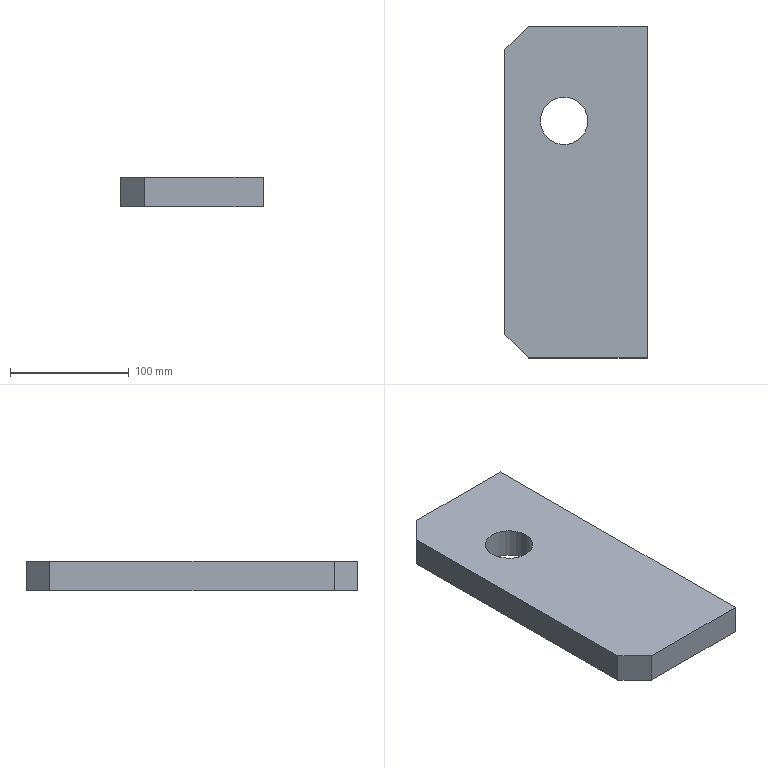Part | SolidWorks | features Chamfer 1, Extrusion 1, ICE 1 | 1 solid | 10 faces | box 120 x 280 x 25 mm | volume 798584 mm3 | plane 8 | cylinder 2 | commonest cylinder face diameters 40 x2
STEP:
#1=CARTESIAN_POINT('',(-90.,200.,0.));
#2=VERTEX_POINT('',#1);
#3=CARTESIAN_POINT('',(-50.,200.,0.));
#4=VERTEX_POINT('',#3);
#5=CARTESIAN_POINT('',(-70.,200.,0.));
#6=DIRECTION('',(0.,0.,1.));
#7=DIRECTION('',(1.,0.,0.));
#8=AXIS2_PLACEMENT_3D('',#5,#6,#7);
#9=CIRCLE('',#8,20.);
#10=EDGE_CURVE('',#2,#4,#9,.T.);
#11=ORIENTED_EDGE('',*,*,#10,.F.);
#12=CARTESIAN_POINT('',(-90.,200.,25.));
#13=VERTEX_POINT('',#12);
#14=CARTESIAN_POINT('',(-90.,200.,0.));
#15=DIRECTION('',(0.,0.,1.));
#16=VECTOR('',#15,1000.);
#17=LINE('',#14,#16);
#18=EDGE_CURVE('',#2,#13,#17,.T.);
#19=ORIENTED_EDGE('',*,*,#18,.T.);
#20=CARTESIAN_POINT('',(-50.,200.,25.));
#21=VERTEX_POINT('',#20);
#22=CARTESIAN_POINT('',(-70.,200.,25.));
#23=DIRECTION('',(0.,0.,1.));
#24=DIRECTION('',(1.,0.,0.));
#25=AXIS2_PLACEMENT_3D('',#22,#23,#24);
#26=CIRCLE('',#25,20.);
#27=EDGE_CURVE('',#13,#21,#26,.T.);
#28=ORIENTED_EDGE('',*,*,#27,.T.);
#29=CARTESIAN_POINT('',(-50.,200.,0.));
#30=DIRECTION('',(0.,0.,1.));
#31=VECTOR('',#30,1000.);
#32=LINE('',#29,#31);
#33=EDGE_CURVE('',#4,#21,#32,.T.);
#34=ORIENTED_EDGE('',*,*,#33,.F.);
#35=EDGE_LOOP('',(#11,#19,#28,#34));
#36=FACE_OUTER_BOUND('',#35,.T.);
#37=CARTESIAN_POINT('',(-70.,200.,0.));
#38=DIRECTION('',(0.,0.,1.));
#39=DIRECTION('',(1.,0.,0.));
#40=AXIS2_PLACEMENT_3D('',#37,#38,#39);
#41=CYLINDRICAL_SURFACE('',#40,20.);
#42=ADVANCED_FACE('',(#36),#41,.F.);
#43=CARTESIAN_POINT('',(0.,0.,0.));
#44=VERTEX_POINT('',#43);
#45=CARTESIAN_POINT('',(0.,280.,0.));
#46=VERTEX_POINT('',#45);
#47=CARTESIAN_POINT('',(0.,0.,0.));
#48=DIRECTION('',(0.,1.,0.));
#49=VECTOR('',#48,1000.);
#50=LINE('',#47,#49);
#51=EDGE_CURVE('',#44,#46,#50,.T.);
#52=ORIENTED_EDGE('',*,*,#51,.T.);
#53=CARTESIAN_POINT('',(0.,280.,25.));
#54=VERTEX_POINT('',#53);
#55=CARTESIAN_POINT('',(0.,280.,25.));
#56=DIRECTION('',(0.,0.,-1.));
#57=VECTOR('',#56,1000.);
#58=LINE('',#55,#57);
#59=EDGE_CURVE('',#54,#46,#58,.T.);
#60=ORIENTED_EDGE('',*,*,#59,.F.);
#61=CARTESIAN_POINT('',(0.,0.,25.));
#62=VERTEX_POINT('',#61);
#63=CARTESIAN_POINT('',(0.,0.,25.));
#64=DIRECTION('',(0.,1.,0.));
#65=VECTOR('',#64,1000.);
#66=LINE('',#63,#65);
#67=EDGE_CURVE('',#62,#54,#66,.T.);
#68=ORIENTED_EDGE('',*,*,#67,.F.);
#69=CARTESIAN_POINT('',(0.,0.,25.));
#70=DIRECTION('',(0.,0.,-1.));
#71=VECTOR('',#70,1000.);
#72=LINE('',#69,#71);
#73=EDGE_CURVE('',#62,#44,#72,.T.);
#74=ORIENTED_EDGE('',*,*,#73,.T.);
#75=EDGE_LOOP('',(#52,#60,#68,#74));
#76=FACE_OUTER_BOUND('',#75,.T.);
#77=CARTESIAN_POINT('',(0.,0.,25.));
#78=DIRECTION('',(-1.,0.,0.));
#79=DIRECTION('',(0.,0.,1.));
#80=AXIS2_PLACEMENT_3D('',#77,#78,#79);
#81=PLANE('',#80);
#82=ADVANCED_FACE('',(#76),#81,.F.);
#83=CARTESIAN_POINT('',(-100.,280.,0.));
#84=VERTEX_POINT('',#83);
#85=CARTESIAN_POINT('',(0.,280.,0.));
#86=DIRECTION('',(-1.,0.,0.));
#87=VECTOR('',#86,1000.);
#88=LINE('',#85,#87);
#89=EDGE_CURVE('',#46,#84,#88,.T.);
#90=ORIENTED_EDGE('',*,*,#89,.T.);
#91=CARTESIAN_POINT('',(-100.,280.,25.));
#92=VERTEX_POINT('',#91);
#93=CARTESIAN_POINT('',(-100.,280.,25.));
#94=DIRECTION('',(0.,0.,1.));
#95=VECTOR('',#94,1000.);
#96=LINE('',#93,#95);
#97=EDGE_CURVE('',#84,#92,#96,.T.);
#98=ORIENTED_EDGE('',*,*,#97,.T.);
#99=CARTESIAN_POINT('',(0.,280.,25.));
#100=DIRECTION('',(-1.,0.,0.));
#101=VECTOR('',#100,1000.);
#102=LINE('',#99,#101);
#103=EDGE_CURVE('',#54,#92,#102,.T.);
#104=ORIENTED_EDGE('',*,*,#103,.F.);
#105=ORIENTED_EDGE('',*,*,#59,.T.);
#106=EDGE_LOOP('',(#90,#98,#104,#105));
#107=FACE_OUTER_BOUND('',#106,.T.);
#108=CARTESIAN_POINT('',(0.,280.,25.));
#109=DIRECTION('',(0.,-1.,0.));
#110=DIRECTION('',(0.,0.,-1.));
#111=AXIS2_PLACEMENT_3D('',#108,#109,#110);
#112=PLANE('',#111);
#113=ADVANCED_FACE('',(#107),#112,.F.);
#114=CARTESIAN_POINT('',(-120.,260.,0.));
#115=VERTEX_POINT('',#114);
#116=CARTESIAN_POINT('',(-120.,20.,0.));
#117=VERTEX_POINT('',#116);
#118=CARTESIAN_POINT('',(-120.,0.,0.));
#119=DIRECTION('',(0.,-1.,0.));
#120=VECTOR('',#119,1000.);
#121=LINE('',#118,#120);
#122=EDGE_CURVE('',#115,#117,#121,.T.);
#123=ORIENTED_EDGE('',*,*,#122,.T.);
#124=CARTESIAN_POINT('',(-120.,20.,25.));
#125=VERTEX_POINT('',#124);
#126=CARTESIAN_POINT('',(-120.,20.,25.));
#127=DIRECTION('',(0.,0.,1.));
#128=VECTOR('',#127,1000.);
#129=LINE('',#126,#128);
#130=EDGE_CURVE('',#117,#125,#129,.T.);
#131=ORIENTED_EDGE('',*,*,#130,.T.);
#132=CARTESIAN_POINT('',(-120.,260.,25.));
#133=VERTEX_POINT('',#132);
#134=CARTESIAN_POINT('',(-120.,0.,25.));
#135=DIRECTION('',(0.,-1.,0.));
#136=VECTOR('',#135,1000.);
#137=LINE('',#134,#136);
#138=EDGE_CURVE('',#133,#125,#137,.T.);
#139=ORIENTED_EDGE('',*,*,#138,.F.);
#140=CARTESIAN_POINT('',(-120.,260.,25.));
#141=DIRECTION('',(0.,0.,-1.));
#142=VECTOR('',#141,1000.);
#143=LINE('',#140,#142);
#144=EDGE_CURVE('',#133,#115,#143,.T.);
#145=ORIENTED_EDGE('',*,*,#144,.T.);
#146=EDGE_LOOP('',(#123,#131,#139,#145));
#147=FACE_OUTER_BOUND('',#146,.T.);
#148=CARTESIAN_POINT('',(-120.,0.,25.));
#149=DIRECTION('',(1.,0.,0.));
#150=DIRECTION('',(0.,0.,-1.));
#151=AXIS2_PLACEMENT_3D('',#148,#149,#150);
#152=PLANE('',#151);
#153=ADVANCED_FACE('',(#147),#152,.F.);
#154=CARTESIAN_POINT('',(-100.,0.,25.));
#155=VERTEX_POINT('',#154);
#156=CARTESIAN_POINT('',(0.,0.,25.));
#157=DIRECTION('',(1.,0.,0.));
#158=VECTOR('',#157,1000.);
#159=LINE('',#156,#158);
#160=EDGE_CURVE('',#155,#62,#159,.T.);
#161=ORIENTED_EDGE('',*,*,#160,.F.);
#162=CARTESIAN_POINT('',(-100.,0.,0.));
#163=VERTEX_POINT('',#162);
#164=CARTESIAN_POINT('',(-100.,0.,25.));
#165=DIRECTION('',(0.,0.,-1.));
#166=VECTOR('',#165,1000.);
#167=LINE('',#164,#166);
#168=EDGE_CURVE('',#155,#163,#167,.T.);
#169=ORIENTED_EDGE('',*,*,#168,.T.);
#170=CARTESIAN_POINT('',(0.,0.,0.));
#171=DIRECTION('',(1.,0.,0.));
#172=VECTOR('',#171,1000.);
#173=LINE('',#170,#172);
#174=EDGE_CURVE('',#163,#44,#173,.T.);
#175=ORIENTED_EDGE('',*,*,#174,.T.);
#176=ORIENTED_EDGE('',*,*,#73,.F.);
#177=EDGE_LOOP('',(#161,#169,#175,#176));
#178=FACE_OUTER_BOUND('',#177,.T.);
#179=CARTESIAN_POINT('',(0.,0.,25.));
#180=DIRECTION('',(0.,1.,0.));
#181=DIRECTION('',(0.,0.,1.));
#182=AXIS2_PLACEMENT_3D('',#179,#180,#181);
#183=PLANE('',#182);
#184=ADVANCED_FACE('',(#178),#183,.F.);
#185=CARTESIAN_POINT('',(-70.,200.,25.));
#186=DIRECTION('',(0.,0.,1.));
#187=DIRECTION('',(1.,0.,0.));
#188=AXIS2_PLACEMENT_3D('',#185,#186,#187);
#189=CIRCLE('',#188,20.);
#190=EDGE_CURVE('',#21,#13,#189,.T.);
#191=ORIENTED_EDGE('',*,*,#190,.F.);
#192=ORIENTED_EDGE('',*,*,#27,.F.);
#193=EDGE_LOOP('',(#191,#192));
#194=FACE_BOUND('',#193,.T.);
#195=ORIENTED_EDGE('',*,*,#138,.T.);
#196=CARTESIAN_POINT('',(-50.,-50.,25.));
#197=DIRECTION('',(0.7071,-0.7071,0.));
#198=VECTOR('',#197,1000.);
#199=LINE('',#196,#198);
#200=EDGE_CURVE('',#125,#155,#199,.T.);
#201=ORIENTED_EDGE('',*,*,#200,.T.);
#202=ORIENTED_EDGE('',*,*,#160,.T.);
#203=ORIENTED_EDGE('',*,*,#67,.T.);
#204=ORIENTED_EDGE('',*,*,#103,.T.);
#205=CARTESIAN_POINT('',(-190.,190.,25.));
#206=DIRECTION('',(-0.7071,-0.7071,0.));
#207=VECTOR('',#206,1000.);
#208=LINE('',#205,#207);
#209=EDGE_CURVE('',#92,#133,#208,.T.);
#210=ORIENTED_EDGE('',*,*,#209,.T.);
#211=EDGE_LOOP('',(#195,#201,#202,#203,#204,#210));
#212=FACE_OUTER_BOUND('',#211,.T.);
#213=CARTESIAN_POINT('',(0.,0.,25.));
#214=DIRECTION('',(0.,0.,1.));
#215=DIRECTION('',(1.,0.,0.));
#216=AXIS2_PLACEMENT_3D('',#213,#214,#215);
#217=PLANE('',#216);
#218=ADVANCED_FACE('',(#194,#212),#217,.T.);
#219=CARTESIAN_POINT('',(-70.,200.,0.));
#220=DIRECTION('',(0.,0.,1.));
#221=DIRECTION('',(1.,0.,0.));
#222=AXIS2_PLACEMENT_3D('',#219,#220,#221);
#223=CIRCLE('',#222,20.);
#224=EDGE_CURVE('',#4,#2,#223,.T.);
#225=ORIENTED_EDGE('',*,*,#224,.T.);
#226=ORIENTED_EDGE('',*,*,#10,.T.);
#227=EDGE_LOOP('',(#225,#226));
#228=FACE_BOUND('',#227,.T.);
#229=ORIENTED_EDGE('',*,*,#174,.F.);
#230=CARTESIAN_POINT('',(-100.,0.,0.));
#231=DIRECTION('',(-0.7071,0.7071,0.));
#232=VECTOR('',#231,1000.);
#233=LINE('',#230,#232);
#234=EDGE_CURVE('',#163,#117,#233,.T.);
#235=ORIENTED_EDGE('',*,*,#234,.T.);
#236=ORIENTED_EDGE('',*,*,#122,.F.);
#237=CARTESIAN_POINT('',(-120.,260.,0.));
#238=DIRECTION('',(0.7071,0.7071,0.));
#239=VECTOR('',#238,1000.);
#240=LINE('',#237,#239);
#241=EDGE_CURVE('',#115,#84,#240,.T.);
#242=ORIENTED_EDGE('',*,*,#241,.T.);
#243=ORIENTED_EDGE('',*,*,#89,.F.);
#244=ORIENTED_EDGE('',*,*,#51,.F.);
#245=EDGE_LOOP('',(#229,#235,#236,#242,#243,#244));
#246=FACE_OUTER_BOUND('',#245,.T.);
#247=CARTESIAN_POINT('',(0.,0.,0.));
#248=DIRECTION('',(0.,0.,1.));
#249=DIRECTION('',(1.,0.,0.));
#250=AXIS2_PLACEMENT_3D('',#247,#248,#249);
#251=PLANE('',#250);
#252=ADVANCED_FACE('',(#228,#246),#251,.F.);
#253=ORIENTED_EDGE('',*,*,#18,.F.);
#254=ORIENTED_EDGE('',*,*,#224,.F.);
#255=ORIENTED_EDGE('',*,*,#33,.T.);
#256=ORIENTED_EDGE('',*,*,#190,.T.);
#257=EDGE_LOOP('',(#253,#254,#255,#256));
#258=FACE_OUTER_BOUND('',#257,.T.);
#259=CARTESIAN_POINT('',(-70.,200.,0.));
#260=DIRECTION('',(0.,0.,1.));
#261=DIRECTION('',(1.,0.,0.));
#262=AXIS2_PLACEMENT_3D('',#259,#260,#261);
#263=CYLINDRICAL_SURFACE('',#262,20.);
#264=ADVANCED_FACE('',(#258),#263,.F.);
#265=ORIENTED_EDGE('',*,*,#200,.F.);
#266=ORIENTED_EDGE('',*,*,#130,.F.);
#267=ORIENTED_EDGE('',*,*,#234,.F.);
#268=ORIENTED_EDGE('',*,*,#168,.F.);
#269=EDGE_LOOP('',(#265,#266,#267,#268));
#270=FACE_OUTER_BOUND('',#269,.T.);
#271=CARTESIAN_POINT('',(-100.,0.,25.));
#272=DIRECTION('',(0.7071,0.7071,0.));
#273=DIRECTION('',(0.,0.,-1.));
#274=AXIS2_PLACEMENT_3D('',#271,#272,#273);
#275=PLANE('',#274);
#276=ADVANCED_FACE('',(#270),#275,.F.);
#277=ORIENTED_EDGE('',*,*,#209,.F.);
#278=ORIENTED_EDGE('',*,*,#97,.F.);
#279=ORIENTED_EDGE('',*,*,#241,.F.);
#280=ORIENTED_EDGE('',*,*,#144,.F.);
#281=EDGE_LOOP('',(#277,#278,#279,#280));
#282=FACE_OUTER_BOUND('',#281,.T.);
#283=CARTESIAN_POINT('',(-120.,260.,25.));
#284=DIRECTION('',(0.7071,-0.7071,0.));
#285=DIRECTION('',(0.,0.,-1.));
#286=AXIS2_PLACEMENT_3D('',#283,#284,#285);
#287=PLANE('',#286);
#288=ADVANCED_FACE('',(#282),#287,.F.);
#289=CLOSED_SHELL('',(#42,#82,#113,#153,#184,#218,#252,#264,#276,#288));
#290=MANIFOLD_SOLID_BREP('',#289);
#291=CARTESIAN_POINT('',(0.,0.,0.));
#292=DIRECTION('',(0.,0.,1.));
#293=DIRECTION('',(1.,0.,0.));
#294=AXIS2_PLACEMENT_3D('',#291,#292,#293);
#295=(LENGTH_UNIT()NAMED_UNIT(*)SI_UNIT(.MILLI.,.METRE.));
#296=UNCERTAINTY_MEASURE_WITH_UNIT(LENGTH_MEASURE(0.00001),#295,'','');
#297=(NAMED_UNIT(*)PLANE_ANGLE_UNIT()SI_UNIT($,.RADIAN.));
#298=(NAMED_UNIT(*)SI_UNIT($,.STERADIAN.)SOLID_ANGLE_UNIT());
#299=(GEOMETRIC_REPRESENTATION_CONTEXT(3)GLOBAL_UNCERTAINTY_ASSIGNED_CONTEXT((#296))GLOBAL_UNIT_ASSIGNED_CONTEXT((#295,#297,#298))REPRESENTATION_CONTEXT('',''));
#300=ADVANCED_BREP_SHAPE_REPRESENTATION('',(#290,#294),#299);